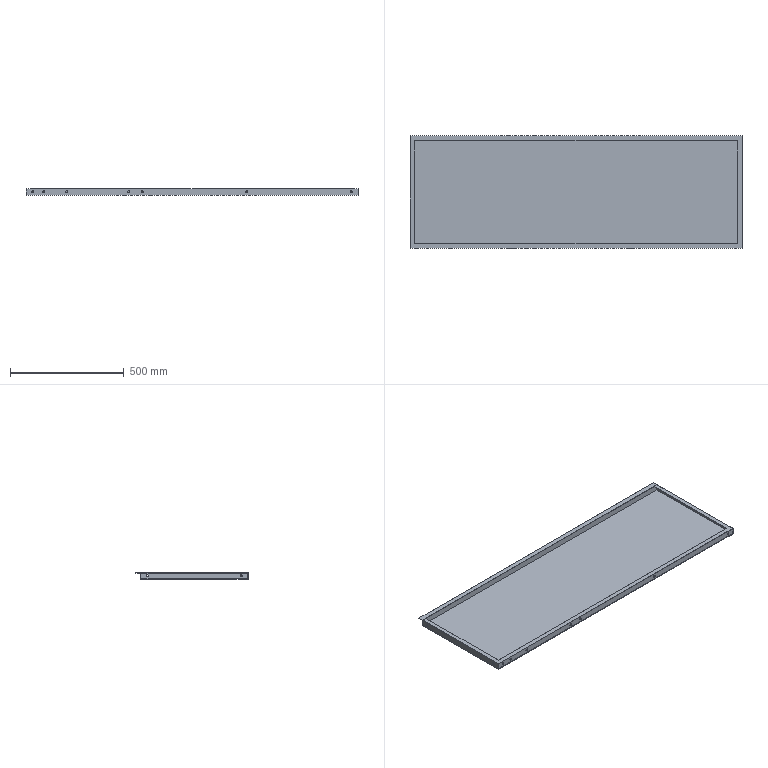Part | SolidWorks | features ICE 3, Extrusion 1, Shell 1 | 1 solid | 39 faces | box 1457 x 492 x 30 mm | volume 1732596 mm3 | cylinder 22 | plane 17 | commonest cylinder face diameters 9 x22
STEP:
#1=CARTESIAN_POINT('',(178.,0.,11.5));
#2=VERTEX_POINT('',#1);
#3=CARTESIAN_POINT('',(178.,0.,20.5));
#4=VERTEX_POINT('',#3);
#5=CARTESIAN_POINT('',(178.,0.,16.));
#6=DIRECTION('',(0.,1.,0.));
#7=DIRECTION('',(0.,0.,1.));
#8=AXIS2_PLACEMENT_3D('',#5,#6,#7);
#9=CIRCLE('',#8,4.5);
#10=EDGE_CURVE('',#2,#4,#9,.T.);
#11=ORIENTED_EDGE('',*,*,#10,.F.);
#12=CARTESIAN_POINT('',(178.,2.,11.5));
#13=VERTEX_POINT('',#12);
#14=CARTESIAN_POINT('',(178.,-8.,11.5));
#15=DIRECTION('',(0.,1.,0.));
#16=VECTOR('',#15,1000.);
#17=LINE('',#14,#16);
#18=EDGE_CURVE('',#2,#13,#17,.T.);
#19=ORIENTED_EDGE('',*,*,#18,.T.);
#20=CARTESIAN_POINT('',(178.,2.,20.5));
#21=VERTEX_POINT('',#20);
#22=CARTESIAN_POINT('',(178.,2.,16.));
#23=DIRECTION('',(0.,1.,0.));
#24=DIRECTION('',(0.,0.,1.));
#25=AXIS2_PLACEMENT_3D('',#22,#23,#24);
#26=CIRCLE('',#25,4.5);
#27=EDGE_CURVE('',#13,#21,#26,.T.);
#28=ORIENTED_EDGE('',*,*,#27,.T.);
#29=CARTESIAN_POINT('',(178.,-8.,20.5));
#30=DIRECTION('',(0.,1.,0.));
#31=VECTOR('',#30,1000.);
#32=LINE('',#29,#31);
#33=EDGE_CURVE('',#4,#21,#32,.T.);
#34=ORIENTED_EDGE('',*,*,#33,.F.);
#35=EDGE_LOOP('',(#11,#19,#28,#34));
#36=FACE_OUTER_BOUND('',#35,.T.);
#37=CARTESIAN_POINT('',(178.,-8.,16.));
#38=DIRECTION('',(0.,1.,0.));
#39=DIRECTION('',(0.,0.,1.));
#40=AXIS2_PLACEMENT_3D('',#37,#38,#39);
#41=CYLINDRICAL_SURFACE('',#40,4.5);
#42=ADVANCED_FACE('',(#36),#41,.F.);
#43=CARTESIAN_POINT('',(78.,0.,11.5));
#44=VERTEX_POINT('',#43);
#45=CARTESIAN_POINT('',(78.,0.,20.5));
#46=VERTEX_POINT('',#45);
#47=CARTESIAN_POINT('',(78.,0.,16.));
#48=DIRECTION('',(0.,1.,0.));
#49=DIRECTION('',(0.,0.,1.));
#50=AXIS2_PLACEMENT_3D('',#47,#48,#49);
#51=CIRCLE('',#50,4.5);
#52=EDGE_CURVE('',#44,#46,#51,.T.);
#53=ORIENTED_EDGE('',*,*,#52,.F.);
#54=CARTESIAN_POINT('',(78.,2.,11.5));
#55=VERTEX_POINT('',#54);
#56=CARTESIAN_POINT('',(78.,-8.,11.5));
#57=DIRECTION('',(0.,1.,0.));
#58=VECTOR('',#57,1000.);
#59=LINE('',#56,#58);
#60=EDGE_CURVE('',#44,#55,#59,.T.);
#61=ORIENTED_EDGE('',*,*,#60,.T.);
#62=CARTESIAN_POINT('',(78.,2.,20.5));
#63=VERTEX_POINT('',#62);
#64=CARTESIAN_POINT('',(78.,2.,16.));
#65=DIRECTION('',(0.,1.,0.));
#66=DIRECTION('',(0.,0.,1.));
#67=AXIS2_PLACEMENT_3D('',#64,#65,#66);
#68=CIRCLE('',#67,4.5);
#69=EDGE_CURVE('',#55,#63,#68,.T.);
#70=ORIENTED_EDGE('',*,*,#69,.T.);
#71=CARTESIAN_POINT('',(78.,-8.,20.5));
#72=DIRECTION('',(0.,1.,0.));
#73=VECTOR('',#72,1000.);
#74=LINE('',#71,#73);
#75=EDGE_CURVE('',#46,#63,#74,.T.);
#76=ORIENTED_EDGE('',*,*,#75,.F.);
#77=EDGE_LOOP('',(#53,#61,#70,#76));
#78=FACE_OUTER_BOUND('',#77,.T.);
#79=CARTESIAN_POINT('',(78.,-8.,16.));
#80=DIRECTION('',(0.,1.,0.));
#81=DIRECTION('',(0.,0.,1.));
#82=AXIS2_PLACEMENT_3D('',#79,#80,#81);
#83=CYLINDRICAL_SURFACE('',#82,4.5);
#84=ADVANCED_FACE('',(#78),#83,.F.);
#85=CARTESIAN_POINT('',(510.,0.,11.5));
#86=VERTEX_POINT('',#85);
#87=CARTESIAN_POINT('',(510.,0.,20.5));
#88=VERTEX_POINT('',#87);
#89=CARTESIAN_POINT('',(510.,0.,16.));
#90=DIRECTION('',(0.,1.,0.));
#91=DIRECTION('',(0.,0.,1.));
#92=AXIS2_PLACEMENT_3D('',#89,#90,#91);
#93=CIRCLE('',#92,4.5);
#94=EDGE_CURVE('',#86,#88,#93,.T.);
#95=ORIENTED_EDGE('',*,*,#94,.F.);
#96=CARTESIAN_POINT('',(510.,2.,11.5));
#97=VERTEX_POINT('',#96);
#98=CARTESIAN_POINT('',(510.,-8.,11.5));
#99=DIRECTION('',(0.,1.,0.));
#100=VECTOR('',#99,1000.);
#101=LINE('',#98,#100);
#102=EDGE_CURVE('',#86,#97,#101,.T.);
#103=ORIENTED_EDGE('',*,*,#102,.T.);
#104=CARTESIAN_POINT('',(510.,2.,20.5));
#105=VERTEX_POINT('',#104);
#106=CARTESIAN_POINT('',(510.,2.,16.));
#107=DIRECTION('',(0.,1.,0.));
#108=DIRECTION('',(0.,0.,1.));
#109=AXIS2_PLACEMENT_3D('',#106,#107,#108);
#110=CIRCLE('',#109,4.5);
#111=EDGE_CURVE('',#97,#105,#110,.T.);
#112=ORIENTED_EDGE('',*,*,#111,.T.);
#113=CARTESIAN_POINT('',(510.,-8.,20.5));
#114=DIRECTION('',(0.,1.,0.));
#115=VECTOR('',#114,1000.);
#116=LINE('',#113,#115);
#117=EDGE_CURVE('',#88,#105,#116,.T.);
#118=ORIENTED_EDGE('',*,*,#117,.F.);
#119=EDGE_LOOP('',(#95,#103,#112,#118));
#120=FACE_OUTER_BOUND('',#119,.T.);
#121=CARTESIAN_POINT('',(510.,-8.,16.));
#122=DIRECTION('',(0.,1.,0.));
#123=DIRECTION('',(0.,0.,1.));
#124=AXIS2_PLACEMENT_3D('',#121,#122,#123);
#125=CYLINDRICAL_SURFACE('',#124,4.5);
#126=ADVANCED_FACE('',(#120),#125,.F.);
#127=CARTESIAN_POINT('',(968.5,0.,11.5));
#128=VERTEX_POINT('',#127);
#129=CARTESIAN_POINT('',(968.5,0.,20.5));
#130=VERTEX_POINT('',#129);
#131=CARTESIAN_POINT('',(968.5,0.,16.));
#132=DIRECTION('',(0.,1.,0.));
#133=DIRECTION('',(0.,0.,1.));
#134=AXIS2_PLACEMENT_3D('',#131,#132,#133);
#135=CIRCLE('',#134,4.5);
#136=EDGE_CURVE('',#128,#130,#135,.T.);
#137=ORIENTED_EDGE('',*,*,#136,.F.);
#138=CARTESIAN_POINT('',(968.5,2.,11.5));
#139=VERTEX_POINT('',#138);
#140=CARTESIAN_POINT('',(968.5,-8.,11.5));
#141=DIRECTION('',(0.,1.,0.));
#142=VECTOR('',#141,1000.);
#143=LINE('',#140,#142);
#144=EDGE_CURVE('',#128,#139,#143,.T.);
#145=ORIENTED_EDGE('',*,*,#144,.T.);
#146=CARTESIAN_POINT('',(968.5,2.,20.5));
#147=VERTEX_POINT('',#146);
#148=CARTESIAN_POINT('',(968.5,2.,16.));
#149=DIRECTION('',(0.,1.,0.));
#150=DIRECTION('',(0.,0.,1.));
#151=AXIS2_PLACEMENT_3D('',#148,#149,#150);
#152=CIRCLE('',#151,4.5);
#153=EDGE_CURVE('',#139,#147,#152,.T.);
#154=ORIENTED_EDGE('',*,*,#153,.T.);
#155=CARTESIAN_POINT('',(968.5,-8.,20.5));
#156=DIRECTION('',(0.,1.,0.));
#157=VECTOR('',#156,1000.);
#158=LINE('',#155,#157);
#159=EDGE_CURVE('',#130,#147,#158,.T.);
#160=ORIENTED_EDGE('',*,*,#159,.F.);
#161=EDGE_LOOP('',(#137,#145,#154,#160));
#162=FACE_OUTER_BOUND('',#161,.T.);
#163=CARTESIAN_POINT('',(968.5,-8.,16.));
#164=DIRECTION('',(0.,1.,0.));
#165=DIRECTION('',(0.,0.,1.));
#166=AXIS2_PLACEMENT_3D('',#163,#164,#165);
#167=CYLINDRICAL_SURFACE('',#166,4.5);
#168=ADVANCED_FACE('',(#162),#167,.F.);
#169=CARTESIAN_POINT('',(1427.,0.,11.5));
#170=VERTEX_POINT('',#169);
#171=CARTESIAN_POINT('',(1427.,0.,20.5));
#172=VERTEX_POINT('',#171);
#173=CARTESIAN_POINT('',(1427.,0.,16.));
#174=DIRECTION('',(0.,1.,0.));
#175=DIRECTION('',(0.,0.,1.));
#176=AXIS2_PLACEMENT_3D('',#173,#174,#175);
#177=CIRCLE('',#176,4.5);
#178=EDGE_CURVE('',#170,#172,#177,.T.);
#179=ORIENTED_EDGE('',*,*,#178,.F.);
#180=CARTESIAN_POINT('',(1427.,2.,11.5));
#181=VERTEX_POINT('',#180);
#182=CARTESIAN_POINT('',(1427.,-8.,11.5));
#183=DIRECTION('',(0.,1.,0.));
#184=VECTOR('',#183,1000.);
#185=LINE('',#182,#184);
#186=EDGE_CURVE('',#170,#181,#185,.T.);
#187=ORIENTED_EDGE('',*,*,#186,.T.);
#188=CARTESIAN_POINT('',(1427.,2.,20.5));
#189=VERTEX_POINT('',#188);
#190=CARTESIAN_POINT('',(1427.,2.,16.));
#191=DIRECTION('',(0.,1.,0.));
#192=DIRECTION('',(0.,0.,1.));
#193=AXIS2_PLACEMENT_3D('',#190,#191,#192);
#194=CIRCLE('',#193,4.5);
#195=EDGE_CURVE('',#181,#189,#194,.T.);
#196=ORIENTED_EDGE('',*,*,#195,.T.);
#197=CARTESIAN_POINT('',(1427.,-8.,20.5));
#198=DIRECTION('',(0.,1.,0.));
#199=VECTOR('',#198,1000.);
#200=LINE('',#197,#199);
#201=EDGE_CURVE('',#172,#189,#200,.T.);
#202=ORIENTED_EDGE('',*,*,#201,.F.);
#203=EDGE_LOOP('',(#179,#187,#196,#202));
#204=FACE_OUTER_BOUND('',#203,.T.);
#205=CARTESIAN_POINT('',(1427.,-8.,16.));
#206=DIRECTION('',(0.,1.,0.));
#207=DIRECTION('',(0.,0.,1.));
#208=AXIS2_PLACEMENT_3D('',#205,#206,#207);
#209=CYLINDRICAL_SURFACE('',#208,4.5);
#210=ADVANCED_FACE('',(#204),#209,.F.);
#211=CARTESIAN_POINT('',(450.,0.,11.5));
#212=VERTEX_POINT('',#211);
#213=CARTESIAN_POINT('',(450.,0.,20.5));
#214=VERTEX_POINT('',#213);
#215=CARTESIAN_POINT('',(450.,0.,16.));
#216=DIRECTION('',(0.,1.,0.));
#217=DIRECTION('',(0.,0.,1.));
#218=AXIS2_PLACEMENT_3D('',#215,#216,#217);
#219=CIRCLE('',#218,4.5);
#220=EDGE_CURVE('',#212,#214,#219,.T.);
#221=ORIENTED_EDGE('',*,*,#220,.F.);
#222=CARTESIAN_POINT('',(450.,2.,11.5));
#223=VERTEX_POINT('',#222);
#224=CARTESIAN_POINT('',(450.,-8.,11.5));
#225=DIRECTION('',(0.,1.,0.));
#226=VECTOR('',#225,1000.);
#227=LINE('',#224,#226);
#228=EDGE_CURVE('',#212,#223,#227,.T.);
#229=ORIENTED_EDGE('',*,*,#228,.T.);
#230=CARTESIAN_POINT('',(450.,2.,20.5));
#231=VERTEX_POINT('',#230);
#232=CARTESIAN_POINT('',(450.,2.,16.));
#233=DIRECTION('',(0.,1.,0.));
#234=DIRECTION('',(0.,0.,1.));
#235=AXIS2_PLACEMENT_3D('',#232,#233,#234);
#236=CIRCLE('',#235,4.5);
#237=EDGE_CURVE('',#223,#231,#236,.T.);
#238=ORIENTED_EDGE('',*,*,#237,.T.);
#239=CARTESIAN_POINT('',(450.,-8.,20.5));
#240=DIRECTION('',(0.,1.,0.));
#241=VECTOR('',#240,1000.);
#242=LINE('',#239,#241);
#243=EDGE_CURVE('',#214,#231,#242,.T.);
#244=ORIENTED_EDGE('',*,*,#243,.F.);
#245=EDGE_LOOP('',(#221,#229,#238,#244));
#246=FACE_OUTER_BOUND('',#245,.T.);
#247=CARTESIAN_POINT('',(450.,-8.,16.));
#248=DIRECTION('',(0.,1.,0.));
#249=DIRECTION('',(0.,0.,1.));
#250=AXIS2_PLACEMENT_3D('',#247,#248,#249);
#251=CYLINDRICAL_SURFACE('',#250,4.5);
#252=ADVANCED_FACE('',(#246),#251,.F.);
#253=CARTESIAN_POINT('',(30.,0.,11.5));
#254=VERTEX_POINT('',#253);
#255=CARTESIAN_POINT('',(30.,0.,20.5));
#256=VERTEX_POINT('',#255);
#257=CARTESIAN_POINT('',(30.,0.,16.));
#258=DIRECTION('',(0.,1.,0.));
#259=DIRECTION('',(0.,0.,1.));
#260=AXIS2_PLACEMENT_3D('',#257,#258,#259);
#261=CIRCLE('',#260,4.5);
#262=EDGE_CURVE('',#254,#256,#261,.T.);
#263=ORIENTED_EDGE('',*,*,#262,.F.);
#264=CARTESIAN_POINT('',(30.,2.,11.5));
#265=VERTEX_POINT('',#264);
#266=CARTESIAN_POINT('',(30.,-8.,11.5));
#267=DIRECTION('',(0.,1.,0.));
#268=VECTOR('',#267,1000.);
#269=LINE('',#266,#268);
#270=EDGE_CURVE('',#254,#265,#269,.T.);
#271=ORIENTED_EDGE('',*,*,#270,.T.);
#272=CARTESIAN_POINT('',(30.,2.,20.5));
#273=VERTEX_POINT('',#272);
#274=CARTESIAN_POINT('',(30.,2.,16.));
#275=DIRECTION('',(0.,1.,0.));
#276=DIRECTION('',(0.,0.,1.));
#277=AXIS2_PLACEMENT_3D('',#274,#275,#276);
#278=CIRCLE('',#277,4.5);
#279=EDGE_CURVE('',#265,#273,#278,.T.);
#280=ORIENTED_EDGE('',*,*,#279,.T.);
#281=CARTESIAN_POINT('',(30.,-8.,20.5));
#282=DIRECTION('',(0.,1.,0.));
#283=VECTOR('',#282,1000.);
#284=LINE('',#281,#283);
#285=EDGE_CURVE('',#256,#273,#284,.T.);
#286=ORIENTED_EDGE('',*,*,#285,.F.);
#287=EDGE_LOOP('',(#263,#271,#280,#286));
#288=FACE_OUTER_BOUND('',#287,.T.);
#289=CARTESIAN_POINT('',(30.,-8.,16.));
#290=DIRECTION('',(0.,1.,0.));
#291=DIRECTION('',(0.,0.,1.));
#292=AXIS2_PLACEMENT_3D('',#289,#290,#291);
#293=CYLINDRICAL_SURFACE('',#292,4.5);
#294=ADVANCED_FACE('',(#288),#293,.F.);
#295=CARTESIAN_POINT('',(2.,30.,11.5));
#296=VERTEX_POINT('',#295);
#297=CARTESIAN_POINT('',(2.,30.,20.5));
#298=VERTEX_POINT('',#297);
#299=CARTESIAN_POINT('',(2.,30.,16.));
#300=DIRECTION('',(-1.,0.,0.));
#301=DIRECTION('',(0.,0.,-1.));
#302=AXIS2_PLACEMENT_3D('',#299,#300,#301);
#303=CIRCLE('',#302,4.5);
#304=EDGE_CURVE('',#296,#298,#303,.T.);
#305=ORIENTED_EDGE('',*,*,#304,.F.);
#306=CARTESIAN_POINT('',(0.,30.,11.5));
#307=VERTEX_POINT('',#306);
#308=CARTESIAN_POINT('',(1503.,30.,11.5));
#309=DIRECTION('',(-1.,0.,0.));
#310=VECTOR('',#309,1000.);
#311=LINE('',#308,#310);
#312=EDGE_CURVE('',#296,#307,#311,.T.);
#313=ORIENTED_EDGE('',*,*,#312,.T.);
#314=CARTESIAN_POINT('',(0.,30.,20.5));
#315=VERTEX_POINT('',#314);
#316=CARTESIAN_POINT('',(0.,30.,16.));
#317=DIRECTION('',(-1.,0.,0.));
#318=DIRECTION('',(0.,0.,-1.));
#319=AXIS2_PLACEMENT_3D('',#316,#317,#318);
#320=CIRCLE('',#319,4.5);
#321=EDGE_CURVE('',#307,#315,#320,.T.);
#322=ORIENTED_EDGE('',*,*,#321,.T.);
#323=CARTESIAN_POINT('',(1503.,30.,20.5));
#324=DIRECTION('',(-1.,0.,0.));
#325=VECTOR('',#324,1000.);
#326=LINE('',#323,#325);
#327=EDGE_CURVE('',#298,#315,#326,.T.);
#328=ORIENTED_EDGE('',*,*,#327,.F.);
#329=EDGE_LOOP('',(#305,#313,#322,#328));
#330=FACE_OUTER_BOUND('',#329,.T.);
#331=CARTESIAN_POINT('',(1503.,30.,16.));
#332=DIRECTION('',(-1.,0.,0.));
#333=DIRECTION('',(0.,0.,1.));
#334=AXIS2_PLACEMENT_3D('',#331,#332,#333);
#335=CYLINDRICAL_SURFACE('',#334,4.5);
#336=ADVANCED_FACE('',(#330),#335,.F.);
#337=CARTESIAN_POINT('',(1457.,30.,20.5));
#338=VERTEX_POINT('',#337);
#339=CARTESIAN_POINT('',(1457.,30.,11.5));
#340=VERTEX_POINT('',#339);
#341=CARTESIAN_POINT('',(1457.,30.,16.));
#342=DIRECTION('',(1.,0.,0.));
#343=DIRECTION('',(0.,0.,1.));
#344=AXIS2_PLACEMENT_3D('',#341,#342,#343);
#345=CIRCLE('',#344,4.5);
#346=EDGE_CURVE('',#338,#340,#345,.T.);
#347=ORIENTED_EDGE('',*,*,#346,.T.);
#348=CARTESIAN_POINT('',(1455.,30.,11.5));
#349=VERTEX_POINT('',#348);
#350=CARTESIAN_POINT('',(1503.,30.,11.5));
#351=DIRECTION('',(-1.,0.,0.));
#352=VECTOR('',#351,1000.);
#353=LINE('',#350,#352);
#354=EDGE_CURVE('',#340,#349,#353,.T.);
#355=ORIENTED_EDGE('',*,*,#354,.T.);
#356=CARTESIAN_POINT('',(1455.,30.,20.5));
#357=VERTEX_POINT('',#356);
#358=CARTESIAN_POINT('',(1455.,30.,16.));
#359=DIRECTION('',(1.,0.,0.));
#360=DIRECTION('',(0.,0.,1.));
#361=AXIS2_PLACEMENT_3D('',#358,#359,#360);
#362=CIRCLE('',#361,4.5);
#363=EDGE_CURVE('',#357,#349,#362,.T.);
#364=ORIENTED_EDGE('',*,*,#363,.F.);
#365=CARTESIAN_POINT('',(1503.,30.,20.5));
#366=DIRECTION('',(-1.,0.,0.));
#367=VECTOR('',#366,1000.);
#368=LINE('',#365,#367);
#369=EDGE_CURVE('',#338,#357,#368,.T.);
#370=ORIENTED_EDGE('',*,*,#369,.F.);
#371=EDGE_LOOP('',(#347,#355,#364,#370));
#372=FACE_OUTER_BOUND('',#371,.T.);
#373=CARTESIAN_POINT('',(1503.,30.,16.));
#374=DIRECTION('',(-1.,0.,0.));
#375=DIRECTION('',(0.,0.,1.));
#376=AXIS2_PLACEMENT_3D('',#373,#374,#375);
#377=CYLINDRICAL_SURFACE('',#376,4.5);
#378=ADVANCED_FACE('',(#372),#377,.F.);
#379=CARTESIAN_POINT('',(2.,442.,11.5));
#380=VERTEX_POINT('',#379);
#381=CARTESIAN_POINT('',(2.,442.,20.5));
#382=VERTEX_POINT('',#381);
#383=CARTESIAN_POINT('',(2.,442.,16.));
#384=DIRECTION('',(-1.,0.,0.));
#385=DIRECTION('',(0.,0.,-1.));
#386=AXIS2_PLACEMENT_3D('',#383,#384,#385);
#387=CIRCLE('',#386,4.5);
#388=EDGE_CURVE('',#380,#382,#387,.T.);
#389=ORIENTED_EDGE('',*,*,#388,.F.);
#390=CARTESIAN_POINT('',(0.,442.,11.5));
#391=VERTEX_POINT('',#390);
#392=CARTESIAN_POINT('',(1503.,442.,11.5));
#393=DIRECTION('',(-1.,0.,0.));
#394=VECTOR('',#393,1000.);
#395=LINE('',#392,#394);
#396=EDGE_CURVE('',#380,#391,#395,.T.);
#397=ORIENTED_EDGE('',*,*,#396,.T.);
#398=CARTESIAN_POINT('',(0.,442.,20.5));
#399=VERTEX_POINT('',#398);
#400=CARTESIAN_POINT('',(0.,442.,16.));
#401=DIRECTION('',(-1.,0.,0.));
#402=DIRECTION('',(0.,0.,-1.));
#403=AXIS2_PLACEMENT_3D('',#400,#401,#402);
#404=CIRCLE('',#403,4.5);
#405=EDGE_CURVE('',#391,#399,#404,.T.);
#406=ORIENTED_EDGE('',*,*,#405,.T.);
#407=CARTESIAN_POINT('',(1503.,442.,20.5));
#408=DIRECTION('',(-1.,0.,0.));
#409=VECTOR('',#408,1000.);
#410=LINE('',#407,#409);
#411=EDGE_CURVE('',#382,#399,#410,.T.);
#412=ORIENTED_EDGE('',*,*,#411,.F.);
#413=EDGE_LOOP('',(#389,#397,#406,#412));
#414=FACE_OUTER_BOUND('',#413,.T.);
#415=CARTESIAN_POINT('',(1503.,442.,16.));
#416=DIRECTION('',(-1.,0.,0.));
#417=DIRECTION('',(0.,0.,1.));
#418=AXIS2_PLACEMENT_3D('',#415,#416,#417);
#419=CYLINDRICAL_SURFACE('',#418,4.5);
#420=ADVANCED_FACE('',(#414),#419,.F.);
#421=CARTESIAN_POINT('',(1457.,442.,20.5));
#422=VERTEX_POINT('',#421);
#423=CARTESIAN_POINT('',(1457.,442.,11.5));
#424=VERTEX_POINT('',#423);
#425=CARTESIAN_POINT('',(1457.,442.,16.));
#426=DIRECTION('',(1.,0.,0.));
#427=DIRECTION('',(0.,0.,1.));
#428=AXIS2_PLACEMENT_3D('',#425,#426,#427);
#429=CIRCLE('',#428,4.5);
#430=EDGE_CURVE('',#422,#424,#429,.T.);
#431=ORIENTED_EDGE('',*,*,#430,.T.);
#432=CARTESIAN_POINT('',(1455.,442.,11.5));
#433=VERTEX_POINT('',#432);
#434=CARTESIAN_POINT('',(1503.,442.,11.5));
#435=DIRECTION('',(-1.,0.,0.));
#436=VECTOR('',#435,1000.);
#437=LINE('',#434,#436);
#438=EDGE_CURVE('',#424,#433,#437,.T.);
#439=ORIENTED_EDGE('',*,*,#438,.T.);
#440=CARTESIAN_POINT('',(1455.,442.,20.5));
#441=VERTEX_POINT('',#440);
#442=CARTESIAN_POINT('',(1455.,442.,16.));
#443=DIRECTION('',(1.,0.,0.));
#444=DIRECTION('',(0.,0.,1.));
#445=AXIS2_PLACEMENT_3D('',#442,#443,#444);
#446=CIRCLE('',#445,4.5);
#447=EDGE_CURVE('',#441,#433,#446,.T.);
#448=ORIENTED_EDGE('',*,*,#447,.F.);
#449=CARTESIAN_POINT('',(1503.,442.,20.5));
#450=DIRECTION('',(-1.,0.,0.));
#451=VECTOR('',#450,1000.);
#452=LINE('',#449,#451);
#453=EDGE_CURVE('',#422,#441,#452,.T.);
#454=ORIENTED_EDGE('',*,*,#453,.F.);
#455=EDGE_LOOP('',(#431,#439,#448,#454));
#456=FACE_OUTER_BOUND('',#455,.T.);
#457=CARTESIAN_POINT('',(1503.,442.,16.));
#458=DIRECTION('',(-1.,0.,0.));
#459=DIRECTION('',(0.,0.,1.));
#460=AXIS2_PLACEMENT_3D('',#457,#458,#459);
#461=CYLINDRICAL_SURFACE('',#460,4.5);
#462=ADVANCED_FACE('',(#456),#461,.F.);
#463=CARTESIAN_POINT('',(2.,442.,16.));
#464=DIRECTION('',(-1.,0.,0.));
#465=DIRECTION('',(0.,0.,-1.));
#466=AXIS2_PLACEMENT_3D('',#463,#464,#465);
#467=CIRCLE('',#466,4.5);
#468=EDGE_CURVE('',#382,#380,#467,.T.);
#469=ORIENTED_EDGE('',*,*,#468,.T.);
#470=ORIENTED_EDGE('',*,*,#388,.T.);
#471=EDGE_LOOP('',(#469,#470));
#472=FACE_BOUND('',#471,.T.);
#473=CARTESIAN_POINT('',(2.,470.,28.));
#474=VERTEX_POINT('',#473);
#475=CARTESIAN_POINT('',(2.,470.,2.));
#476=VERTEX_POINT('',#475);
#477=CARTESIAN_POINT('',(2.,470.,30.));
#478=DIRECTION('',(0.,0.,-1.));
#479=VECTOR('',#478,1000.);
#480=LINE('',#477,#479);
#481=EDGE_CURVE('',#474,#476,#480,.T.);
#482=ORIENTED_EDGE('',*,*,#481,.F.);
#483=CARTESIAN_POINT('',(2.,2.,28.));
#484=VERTEX_POINT('',#483);
#485=CARTESIAN_POINT('',(2.,0.,28.));
#486=DIRECTION('',(0.,-1.,0.));
#487=VECTOR('',#486,1000.);
#488=LINE('',#485,#487);
#489=EDGE_CURVE('',#474,#484,#488,.T.);
#490=ORIENTED_EDGE('',*,*,#489,.T.);
#491=CARTESIAN_POINT('',(2.,2.,2.));
#492=VERTEX_POINT('',#491);
#493=CARTESIAN_POINT('',(2.,2.,30.));
#494=DIRECTION('',(0.,0.,-1.));
#495=VECTOR('',#494,1000.);
#496=LINE('',#493,#495);
#497=EDGE_CURVE('',#484,#492,#496,.T.);
#498=ORIENTED_EDGE('',*,*,#497,.T.);
#499=CARTESIAN_POINT('',(2.,472.,2.));
#500=DIRECTION('',(0.,-1.,0.));
#501=VECTOR('',#500,1000.);
#502=LINE('',#499,#501);
#503=EDGE_CURVE('',#476,#492,#502,.T.);
#504=ORIENTED_EDGE('',*,*,#503,.F.);
#505=EDGE_LOOP('',(#482,#490,#498,#504));
#506=FACE_OUTER_BOUND('',#505,.T.);
#507=CARTESIAN_POINT('',(2.,30.,16.));
#508=DIRECTION('',(-1.,0.,0.));
#509=DIRECTION('',(0.,0.,-1.));
#510=AXIS2_PLACEMENT_3D('',#507,#508,#509);
#511=CIRCLE('',#510,4.5);
#512=EDGE_CURVE('',#298,#296,#511,.T.);
#513=ORIENTED_EDGE('',*,*,#512,.T.);
#514=ORIENTED_EDGE('',*,*,#304,.T.);
#515=EDGE_LOOP('',(#513,#514));
#516=FACE_BOUND('',#515,.T.);
#517=CARTESIAN_POINT('',(2.,0.,30.));
#518=DIRECTION('',(1.,0.,0.));
#519=DIRECTION('',(0.,0.,-1.));
#520=AXIS2_PLACEMENT_3D('',#517,#518,#519);
#521=PLANE('',#520);
#522=ADVANCED_FACE('',(#472,#506,#516),#521,.T.);
#523=ORIENTED_EDGE('',*,*,#447,.T.);
#524=CARTESIAN_POINT('',(1455.,442.,16.));
#525=DIRECTION('',(1.,0.,0.));
#526=DIRECTION('',(0.,0.,1.));
#527=AXIS2_PLACEMENT_3D('',#524,#525,#526);
#528=CIRCLE('',#527,4.5);
#529=EDGE_CURVE('',#433,#441,#528,.T.);
#530=ORIENTED_EDGE('',*,*,#529,.T.);
#531=EDGE_LOOP('',(#523,#530));
#532=FACE_BOUND('',#531,.T.);
#533=CARTESIAN_POINT('',(1455.,2.,28.));
#534=VERTEX_POINT('',#533);
#535=CARTESIAN_POINT('',(1455.,2.,2.));
#536=VERTEX_POINT('',#535);
#537=CARTESIAN_POINT('',(1455.,2.,30.));
#538=DIRECTION('',(0.,0.,-1.));
#539=VECTOR('',#538,1000.);
#540=LINE('',#537,#539);
#541=EDGE_CURVE('',#534,#536,#540,.T.);
#542=ORIENTED_EDGE('',*,*,#541,.F.);
#543=CARTESIAN_POINT('',(1455.,470.,28.));
#544=VERTEX_POINT('',#543);
#545=CARTESIAN_POINT('',(1455.,0.,28.));
#546=DIRECTION('',(0.,1.,0.));
#547=VECTOR('',#546,1000.);
#548=LINE('',#545,#547);
#549=EDGE_CURVE('',#534,#544,#548,.T.);
#550=ORIENTED_EDGE('',*,*,#549,.T.);
#551=CARTESIAN_POINT('',(1455.,470.,2.));
#552=VERTEX_POINT('',#551);
#553=CARTESIAN_POINT('',(1455.,470.,30.));
#554=DIRECTION('',(0.,0.,-1.));
#555=VECTOR('',#554,1000.);
#556=LINE('',#553,#555);
#557=EDGE_CURVE('',#544,#552,#556,.T.);
#558=ORIENTED_EDGE('',*,*,#557,.T.);
#559=CARTESIAN_POINT('',(1455.,472.,2.));
#560=DIRECTION('',(0.,1.,0.));
#561=VECTOR('',#560,1000.);
#562=LINE('',#559,#561);
#563=EDGE_CURVE('',#536,#552,#562,.T.);
#564=ORIENTED_EDGE('',*,*,#563,.F.);
#565=EDGE_LOOP('',(#542,#550,#558,#564));
#566=FACE_OUTER_BOUND('',#565,.T.);
#567=ORIENTED_EDGE('',*,*,#363,.T.);
#568=CARTESIAN_POINT('',(1455.,30.,16.));
#569=DIRECTION('',(1.,0.,0.));
#570=DIRECTION('',(0.,0.,1.));
#571=AXIS2_PLACEMENT_3D('',#568,#569,#570);
#572=CIRCLE('',#571,4.5);
#573=EDGE_CURVE('',#349,#357,#572,.T.);
#574=ORIENTED_EDGE('',*,*,#573,.T.);
#575=EDGE_LOOP('',(#567,#574));
#576=FACE_BOUND('',#575,.T.);
#577=CARTESIAN_POINT('',(1455.,0.,30.));
#578=DIRECTION('',(-1.,0.,0.));
#579=DIRECTION('',(0.,0.,1.));
#580=AXIS2_PLACEMENT_3D('',#577,#578,#579);
#581=PLANE('',#580);
#582=ADVANCED_FACE('',(#532,#566,#576),#581,.T.);
#583=CARTESIAN_POINT('',(0.,442.,16.));
#584=DIRECTION('',(-1.,0.,0.));
#585=DIRECTION('',(0.,0.,-1.));
#586=AXIS2_PLACEMENT_3D('',#583,#584,#585);
#587=CIRCLE('',#586,4.5);
#588=EDGE_CURVE('',#399,#391,#587,.T.);
#589=ORIENTED_EDGE('',*,*,#588,.F.);
#590=ORIENTED_EDGE('',*,*,#405,.F.);
#591=EDGE_LOOP('',(#589,#590));
#592=FACE_BOUND('',#591,.T.);
#593=CARTESIAN_POINT('',(0.,492.,30.));
#594=VERTEX_POINT('',#593);
#595=CARTESIAN_POINT('',(0.,0.,30.));
#596=VERTEX_POINT('',#595);
#597=CARTESIAN_POINT('',(0.,0.,30.));
#598=DIRECTION('',(0.,-1.,0.));
#599=VECTOR('',#598,1000.);
#600=LINE('',#597,#599);
#601=EDGE_CURVE('',#594,#596,#600,.T.);
#602=ORIENTED_EDGE('',*,*,#601,.F.);
#603=CARTESIAN_POINT('',(0.,492.,28.));
#604=VERTEX_POINT('',#603);
#605=CARTESIAN_POINT('',(0.,492.,28.));
#606=DIRECTION('',(0.,0.,1.));
#607=VECTOR('',#606,1000.);
#608=LINE('',#605,#607);
#609=EDGE_CURVE('',#604,#594,#608,.T.);
#610=ORIENTED_EDGE('',*,*,#609,.F.);
#611=CARTESIAN_POINT('',(0.,472.,28.));
#612=VERTEX_POINT('',#611);
#613=CARTESIAN_POINT('',(0.,492.,28.));
#614=DIRECTION('',(0.,-1.,0.));
#615=VECTOR('',#614,1000.);
#616=LINE('',#613,#615);
#617=EDGE_CURVE('',#604,#612,#616,.T.);
#618=ORIENTED_EDGE('',*,*,#617,.T.);
#619=CARTESIAN_POINT('',(0.,472.,0.));
#620=VERTEX_POINT('',#619);
#621=CARTESIAN_POINT('',(0.,472.,30.));
#622=DIRECTION('',(0.,0.,-1.));
#623=VECTOR('',#622,1000.);
#624=LINE('',#621,#623);
#625=EDGE_CURVE('',#612,#620,#624,.T.);
#626=ORIENTED_EDGE('',*,*,#625,.T.);
#627=CARTESIAN_POINT('',(0.,0.,0.));
#628=VERTEX_POINT('',#627);
#629=CARTESIAN_POINT('',(0.,0.,0.));
#630=DIRECTION('',(0.,-1.,0.));
#631=VECTOR('',#630,1000.);
#632=LINE('',#629,#631);
#633=EDGE_CURVE('',#620,#628,#632,.T.);
#634=ORIENTED_EDGE('',*,*,#633,.T.);
#635=CARTESIAN_POINT('',(0.,0.,30.));
#636=DIRECTION('',(0.,0.,-1.));
#637=VECTOR('',#636,1000.);
#638=LINE('',#635,#637);
#639=EDGE_CURVE('',#596,#628,#638,.T.);
#640=ORIENTED_EDGE('',*,*,#639,.F.);
#641=EDGE_LOOP('',(#602,#610,#618,#626,#634,#640));
#642=FACE_OUTER_BOUND('',#641,.T.);
#643=CARTESIAN_POINT('',(0.,30.,16.));
#644=DIRECTION('',(-1.,0.,0.));
#645=DIRECTION('',(0.,0.,-1.));
#646=AXIS2_PLACEMENT_3D('',#643,#644,#645);
#647=CIRCLE('',#646,4.5);
#648=EDGE_CURVE('',#315,#307,#647,.T.);
#649=ORIENTED_EDGE('',*,*,#648,.F.);
#650=ORIENTED_EDGE('',*,*,#321,.F.);
#651=EDGE_LOOP('',(#649,#650));
#652=FACE_BOUND('',#651,.T.);
#653=CARTESIAN_POINT('',(0.,0.,30.));
#654=DIRECTION('',(1.,0.,0.));
#655=DIRECTION('',(0.,0.,-1.));
#656=AXIS2_PLACEMENT_3D('',#653,#654,#655);
#657=PLANE('',#656);
#658=ADVANCED_FACE('',(#592,#642,#652),#657,.F.);
#659=ORIENTED_EDGE('',*,*,#430,.F.);
#660=CARTESIAN_POINT('',(1457.,442.,16.));
#661=DIRECTION('',(1.,0.,0.));
#662=DIRECTION('',(0.,0.,1.));
#663=AXIS2_PLACEMENT_3D('',#660,#661,#662);
#664=CIRCLE('',#663,4.5);
#665=EDGE_CURVE('',#424,#422,#664,.T.);
#666=ORIENTED_EDGE('',*,*,#665,.F.);
#667=EDGE_LOOP('',(#659,#666));
#668=FACE_BOUND('',#667,.T.);
#669=CARTESIAN_POINT('',(1457.,0.,30.));
#670=VERTEX_POINT('',#669);
#671=CARTESIAN_POINT('',(1457.,0.,0.));
#672=VERTEX_POINT('',#671);
#673=CARTESIAN_POINT('',(1457.,0.,30.));
#674=DIRECTION('',(0.,0.,-1.));
#675=VECTOR('',#674,1000.);
#676=LINE('',#673,#675);
#677=EDGE_CURVE('',#670,#672,#676,.T.);
#678=ORIENTED_EDGE('',*,*,#677,.T.);
#679=CARTESIAN_POINT('',(1457.,472.,0.));
#680=VERTEX_POINT('',#679);
#681=CARTESIAN_POINT('',(1457.,0.,0.));
#682=DIRECTION('',(0.,1.,0.));
#683=VECTOR('',#682,1000.);
#684=LINE('',#681,#683);
#685=EDGE_CURVE('',#672,#680,#684,.T.);
#686=ORIENTED_EDGE('',*,*,#685,.T.);
#687=CARTESIAN_POINT('',(1457.,472.,28.));
#688=VERTEX_POINT('',#687);
#689=CARTESIAN_POINT('',(1457.,472.,30.));
#690=DIRECTION('',(0.,0.,-1.));
#691=VECTOR('',#690,1000.);
#692=LINE('',#689,#691);
#693=EDGE_CURVE('',#688,#680,#692,.T.);
#694=ORIENTED_EDGE('',*,*,#693,.F.);
#695=CARTESIAN_POINT('',(1457.,492.,28.));
#696=VERTEX_POINT('',#695);
#697=CARTESIAN_POINT('',(1457.,492.,28.));
#698=DIRECTION('',(0.,1.,0.));
#699=VECTOR('',#698,1000.);
#700=LINE('',#697,#699);
#701=EDGE_CURVE('',#688,#696,#700,.T.);
#702=ORIENTED_EDGE('',*,*,#701,.T.);
#703=CARTESIAN_POINT('',(1457.,492.,30.));
#704=VERTEX_POINT('',#703);
#705=CARTESIAN_POINT('',(1457.,492.,28.));
#706=DIRECTION('',(0.,0.,1.));
#707=VECTOR('',#706,1000.);
#708=LINE('',#705,#707);
#709=EDGE_CURVE('',#696,#704,#708,.T.);
#710=ORIENTED_EDGE('',*,*,#709,.T.);
#711=CARTESIAN_POINT('',(1457.,0.,30.));
#712=DIRECTION('',(0.,1.,0.));
#713=VECTOR('',#712,1000.);
#714=LINE('',#711,#713);
#715=EDGE_CURVE('',#670,#704,#714,.T.);
#716=ORIENTED_EDGE('',*,*,#715,.F.);
#717=EDGE_LOOP('',(#678,#686,#694,#702,#710,#716));
#718=FACE_OUTER_BOUND('',#717,.T.);
#719=ORIENTED_EDGE('',*,*,#346,.F.);
#720=CARTESIAN_POINT('',(1457.,30.,16.));
#721=DIRECTION('',(1.,0.,0.));
#722=DIRECTION('',(0.,0.,1.));
#723=AXIS2_PLACEMENT_3D('',#720,#721,#722);
#724=CIRCLE('',#723,4.5);
#725=EDGE_CURVE('',#340,#338,#724,.T.);
#726=ORIENTED_EDGE('',*,*,#725,.F.);
#727=EDGE_LOOP('',(#719,#726));
#728=FACE_BOUND('',#727,.T.);
#729=CARTESIAN_POINT('',(1457.,0.,30.));
#730=DIRECTION('',(-1.,0.,0.));
#731=DIRECTION('',(0.,0.,1.));
#732=AXIS2_PLACEMENT_3D('',#729,#730,#731);
#733=PLANE('',#732);
#734=ADVANCED_FACE('',(#668,#718,#728),#733,.F.);
#735=CARTESIAN_POINT('',(0.,472.,28.));
#736=DIRECTION('',(-1.,0.,0.));
#737=VECTOR('',#736,1000.);
#738=LINE('',#735,#737);
#739=EDGE_CURVE('',#688,#612,#738,.T.);
#740=ORIENTED_EDGE('',*,*,#739,.F.);
#741=ORIENTED_EDGE('',*,*,#693,.T.);
#742=CARTESIAN_POINT('',(0.,472.,0.));
#743=DIRECTION('',(-1.,0.,0.));
#744=VECTOR('',#743,1000.);
#745=LINE('',#742,#744);
#746=EDGE_CURVE('',#680,#620,#745,.T.);
#747=ORIENTED_EDGE('',*,*,#746,.T.);
#748=ORIENTED_EDGE('',*,*,#625,.F.);
#749=EDGE_LOOP('',(#740,#741,#747,#748));
#750=FACE_OUTER_BOUND('',#749,.T.);
#751=CARTESIAN_POINT('',(0.,472.,30.));
#752=DIRECTION('',(0.,-1.,0.));
#753=DIRECTION('',(1.,0.,0.));
#754=AXIS2_PLACEMENT_3D('',#751,#752,#753);
#755=PLANE('',#754);
#756=ADVANCED_FACE('',(#750),#755,.F.);
#757=CARTESIAN_POINT('',(178.,2.,16.));
#758=DIRECTION('',(0.,1.,0.));
#759=DIRECTION('',(0.,0.,1.));
#760=AXIS2_PLACEMENT_3D('',#757,#758,#759);
#761=CIRCLE('',#760,4.5);
#762=EDGE_CURVE('',#21,#13,#761,.T.);
#763=ORIENTED_EDGE('',*,*,#762,.F.);
#764=ORIENTED_EDGE('',*,*,#27,.F.);
#765=EDGE_LOOP('',(#763,#764));
#766=FACE_BOUND('',#765,.T.);
#767=CARTESIAN_POINT('',(78.,2.,16.));
#768=DIRECTION('',(0.,1.,0.));
#769=DIRECTION('',(0.,0.,1.));
#770=AXIS2_PLACEMENT_3D('',#767,#768,#769);
#771=CIRCLE('',#770,4.5);
#772=EDGE_CURVE('',#63,#55,#771,.T.);
#773=ORIENTED_EDGE('',*,*,#772,.F.);
#774=ORIENTED_EDGE('',*,*,#69,.F.);
#775=EDGE_LOOP('',(#773,#774));
#776=FACE_BOUND('',#775,.T.);
#777=CARTESIAN_POINT('',(510.,2.,16.));
#778=DIRECTION('',(0.,1.,0.));
#779=DIRECTION('',(0.,0.,1.));
#780=AXIS2_PLACEMENT_3D('',#777,#778,#779);
#781=CIRCLE('',#780,4.5);
#782=EDGE_CURVE('',#105,#97,#781,.T.);
#783=ORIENTED_EDGE('',*,*,#782,.F.);
#784=ORIENTED_EDGE('',*,*,#111,.F.);
#785=EDGE_LOOP('',(#783,#784));
#786=FACE_BOUND('',#785,.T.);
#787=CARTESIAN_POINT('',(968.5,2.,16.));
#788=DIRECTION('',(0.,1.,0.));
#789=DIRECTION('',(0.,0.,1.));
#790=AXIS2_PLACEMENT_3D('',#787,#788,#789);
#791=CIRCLE('',#790,4.5);
#792=EDGE_CURVE('',#147,#139,#791,.T.);
#793=ORIENTED_EDGE('',*,*,#792,.F.);
#794=ORIENTED_EDGE('',*,*,#153,.F.);
#795=EDGE_LOOP('',(#793,#794));
#796=FACE_BOUND('',#795,.T.);
#797=CARTESIAN_POINT('',(1427.,2.,16.));
#798=DIRECTION('',(0.,1.,0.));
#799=DIRECTION('',(0.,0.,1.));
#800=AXIS2_PLACEMENT_3D('',#797,#798,#799);
#801=CIRCLE('',#800,4.5);
#802=EDGE_CURVE('',#189,#181,#801,.T.);
#803=ORIENTED_EDGE('',*,*,#802,.F.);
#804=ORIENTED_EDGE('',*,*,#195,.F.);
#805=EDGE_LOOP('',(#803,#804));
#806=FACE_BOUND('',#805,.T.);
#807=CARTESIAN_POINT('',(450.,2.,16.));
#808=DIRECTION('',(0.,1.,0.));
#809=DIRECTION('',(0.,0.,1.));
#810=AXIS2_PLACEMENT_3D('',#807,#808,#809);
#811=CIRCLE('',#810,4.5);
#812=EDGE_CURVE('',#231,#223,#811,.T.);
#813=ORIENTED_EDGE('',*,*,#812,.F.);
#814=ORIENTED_EDGE('',*,*,#237,.F.);
#815=EDGE_LOOP('',(#813,#814));
#816=FACE_BOUND('',#815,.T.);
#817=CARTESIAN_POINT('',(30.,2.,16.));
#818=DIRECTION('',(0.,1.,0.));
#819=DIRECTION('',(0.,0.,1.));
#820=AXIS2_PLACEMENT_3D('',#817,#818,#819);
#821=CIRCLE('',#820,4.5);
#822=EDGE_CURVE('',#273,#265,#821,.T.);
#823=ORIENTED_EDGE('',*,*,#822,.F.);
#824=ORIENTED_EDGE('',*,*,#279,.F.);
#825=EDGE_LOOP('',(#823,#824));
#826=FACE_BOUND('',#825,.T.);
#827=ORIENTED_EDGE('',*,*,#497,.F.);
#828=CARTESIAN_POINT('',(0.,2.,28.));
#829=DIRECTION('',(1.,0.,0.));
#830=VECTOR('',#829,1000.);
#831=LINE('',#828,#830);
#832=EDGE_CURVE('',#484,#534,#831,.T.);
#833=ORIENTED_EDGE('',*,*,#832,.T.);
#834=ORIENTED_EDGE('',*,*,#541,.T.);
#835=CARTESIAN_POINT('',(0.,2.,2.));
#836=DIRECTION('',(1.,0.,0.));
#837=VECTOR('',#836,1000.);
#838=LINE('',#835,#837);
#839=EDGE_CURVE('',#492,#536,#838,.T.);
#840=ORIENTED_EDGE('',*,*,#839,.F.);
#841=EDGE_LOOP('',(#827,#833,#834,#840));
#842=FACE_OUTER_BOUND('',#841,.T.);
#843=CARTESIAN_POINT('',(0.,2.,30.));
#844=DIRECTION('',(0.,1.,0.));
#845=DIRECTION('',(0.,0.,1.));
#846=AXIS2_PLACEMENT_3D('',#843,#844,#845);
#847=PLANE('',#846);
#848=ADVANCED_FACE('',(#766,#776,#786,#796,#806,#816,#826,#842),#847,.T.);
#849=CARTESIAN_POINT('',(1437.,470.,30.));
#850=VERTEX_POINT('',#849);
#851=CARTESIAN_POINT('',(20.,470.,30.));
#852=VERTEX_POINT('',#851);
#853=CARTESIAN_POINT('',(0.,470.,30.));
#854=DIRECTION('',(-1.,0.,0.));
#855=VECTOR('',#854,1000.);
#856=LINE('',#853,#855);
#857=EDGE_CURVE('',#850,#852,#856,.T.);
#858=ORIENTED_EDGE('',*,*,#857,.T.);
#859=CARTESIAN_POINT('',(20.,470.,28.));
#860=VERTEX_POINT('',#859);
#861=CARTESIAN_POINT('',(20.,470.,28.));
#862=DIRECTION('',(0.,0.,1.));
#863=VECTOR('',#862,1000.);
#864=LINE('',#861,#863);
#865=EDGE_CURVE('',#860,#852,#864,.T.);
#866=ORIENTED_EDGE('',*,*,#865,.F.);
#867=CARTESIAN_POINT('',(0.,470.,28.));
#868=DIRECTION('',(-1.,0.,0.));
#869=VECTOR('',#868,1000.);
#870=LINE('',#867,#869);
#871=EDGE_CURVE('',#860,#474,#870,.T.);
#872=ORIENTED_EDGE('',*,*,#871,.T.);
#873=ORIENTED_EDGE('',*,*,#481,.T.);
#874=CARTESIAN_POINT('',(0.,470.,2.));
#875=DIRECTION('',(-1.,0.,0.));
#876=VECTOR('',#875,1000.);
#877=LINE('',#874,#876);
#878=EDGE_CURVE('',#552,#476,#877,.T.);
#879=ORIENTED_EDGE('',*,*,#878,.F.);
#880=ORIENTED_EDGE('',*,*,#557,.F.);
#881=CARTESIAN_POINT('',(1437.,470.,28.));
#882=VERTEX_POINT('',#881);
#883=CARTESIAN_POINT('',(0.,470.,28.));
#884=DIRECTION('',(-1.,0.,0.));
#885=VECTOR('',#884,1000.);
#886=LINE('',#883,#885);
#887=EDGE_CURVE('',#544,#882,#886,.T.);
#888=ORIENTED_EDGE('',*,*,#887,.T.);
#889=CARTESIAN_POINT('',(1437.,470.,28.));
#890=DIRECTION('',(0.,0.,1.));
#891=VECTOR('',#890,1000.);
#892=LINE('',#889,#891);
#893=EDGE_CURVE('',#882,#850,#892,.T.);
#894=ORIENTED_EDGE('',*,*,#893,.T.);
#895=EDGE_LOOP('',(#858,#866,#872,#873,#879,#880,#888,#894));
#896=FACE_OUTER_BOUND('',#895,.T.);
#897=CARTESIAN_POINT('',(0.,470.,30.));
#898=DIRECTION('',(0.,-1.,0.));
#899=DIRECTION('',(1.,0.,0.));
#900=AXIS2_PLACEMENT_3D('',#897,#898,#899);
#901=PLANE('',#900);
#902=ADVANCED_FACE('',(#896),#901,.T.);
#903=ORIENTED_EDGE('',*,*,#857,.F.);
#904=CARTESIAN_POINT('',(1437.,20.,30.));
#905=VERTEX_POINT('',#904);
#906=CARTESIAN_POINT('',(1437.,20.,30.));
#907=DIRECTION('',(0.,1.,0.));
#908=VECTOR('',#907,1000.);
#909=LINE('',#906,#908);
#910=EDGE_CURVE('',#905,#850,#909,.T.);
#911=ORIENTED_EDGE('',*,*,#910,.F.);
#912=CARTESIAN_POINT('',(20.,20.,30.));
#913=VERTEX_POINT('',#912);
#914=CARTESIAN_POINT('',(20.,20.,30.));
#915=DIRECTION('',(1.,0.,0.));
#916=VECTOR('',#915,1000.);
#917=LINE('',#914,#916);
#918=EDGE_CURVE('',#913,#905,#917,.T.);
#919=ORIENTED_EDGE('',*,*,#918,.F.);
#920=CARTESIAN_POINT('',(20.,20.,30.));
#921=DIRECTION('',(0.,-1.,0.));
#922=VECTOR('',#921,1000.);
#923=LINE('',#920,#922);
#924=EDGE_CURVE('',#852,#913,#923,.T.);
#925=ORIENTED_EDGE('',*,*,#924,.F.);
#926=EDGE_LOOP('',(#903,#911,#919,#925));
#927=FACE_BOUND('',#926,.T.);
#928=ORIENTED_EDGE('',*,*,#601,.T.);
#929=CARTESIAN_POINT('',(0.,0.,30.));
#930=DIRECTION('',(1.,0.,0.));
#931=VECTOR('',#930,1000.);
#932=LINE('',#929,#931);
#933=EDGE_CURVE('',#596,#670,#932,.T.);
#934=ORIENTED_EDGE('',*,*,#933,.T.);
#935=ORIENTED_EDGE('',*,*,#715,.T.);
#936=CARTESIAN_POINT('',(0.,492.,30.));
#937=DIRECTION('',(-1.,0.,0.));
#938=VECTOR('',#937,1000.);
#939=LINE('',#936,#938);
#940=EDGE_CURVE('',#704,#594,#939,.T.);
#941=ORIENTED_EDGE('',*,*,#940,.T.);
#942=EDGE_LOOP('',(#928,#934,#935,#941));
#943=FACE_OUTER_BOUND('',#942,.T.);
#944=CARTESIAN_POINT('',(0.,472.,30.));
#945=DIRECTION('',(0.,0.,-1.));
#946=DIRECTION('',(-1.,0.,0.));
#947=AXIS2_PLACEMENT_3D('',#944,#945,#946);
#948=PLANE('',#947);
#949=ADVANCED_FACE('',(#927,#943),#948,.F.);
#950=CARTESIAN_POINT('',(178.,0.,16.));
#951=DIRECTION('',(0.,1.,0.));
#952=DIRECTION('',(0.,0.,1.));
#953=AXIS2_PLACEMENT_3D('',#950,#951,#952);
#954=CIRCLE('',#953,4.5);
#955=EDGE_CURVE('',#4,#2,#954,.T.);
#956=ORIENTED_EDGE('',*,*,#955,.T.);
#957=ORIENTED_EDGE('',*,*,#10,.T.);
#958=EDGE_LOOP('',(#956,#957));
#959=FACE_BOUND('',#958,.T.);
#960=CARTESIAN_POINT('',(78.,0.,16.));
#961=DIRECTION('',(0.,1.,0.));
#962=DIRECTION('',(0.,0.,1.));
#963=AXIS2_PLACEMENT_3D('',#960,#961,#962);
#964=CIRCLE('',#963,4.5);
#965=EDGE_CURVE('',#46,#44,#964,.T.);
#966=ORIENTED_EDGE('',*,*,#965,.T.);
#967=ORIENTED_EDGE('',*,*,#52,.T.);
#968=EDGE_LOOP('',(#966,#967));
#969=FACE_BOUND('',#968,.T.);
#970=CARTESIAN_POINT('',(510.,0.,16.));
#971=DIRECTION('',(0.,1.,0.));
#972=DIRECTION('',(0.,0.,1.));
#973=AXIS2_PLACEMENT_3D('',#970,#971,#972);
#974=CIRCLE('',#973,4.5);
#975=EDGE_CURVE('',#88,#86,#974,.T.);
#976=ORIENTED_EDGE('',*,*,#975,.T.);
#977=ORIENTED_EDGE('',*,*,#94,.T.);
#978=EDGE_LOOP('',(#976,#977));
#979=FACE_BOUND('',#978,.T.);
#980=CARTESIAN_POINT('',(968.5,0.,16.));
#981=DIRECTION('',(0.,1.,0.));
#982=DIRECTION('',(0.,0.,1.));
#983=AXIS2_PLACEMENT_3D('',#980,#981,#982);
#984=CIRCLE('',#983,4.5);
#985=EDGE_CURVE('',#130,#128,#984,.T.);
#986=ORIENTED_EDGE('',*,*,#985,.T.);
#987=ORIENTED_EDGE('',*,*,#136,.T.);
#988=EDGE_LOOP('',(#986,#987));
#989=FACE_BOUND('',#988,.T.);
#990=CARTESIAN_POINT('',(1427.,0.,16.));
#991=DIRECTION('',(0.,1.,0.));
#992=DIRECTION('',(0.,0.,1.));
#993=AXIS2_PLACEMENT_3D('',#990,#991,#992);
#994=CIRCLE('',#993,4.5);
#995=EDGE_CURVE('',#172,#170,#994,.T.);
#996=ORIENTED_EDGE('',*,*,#995,.T.);
#997=ORIENTED_EDGE('',*,*,#178,.T.);
#998=EDGE_LOOP('',(#996,#997));
#999=FACE_BOUND('',#998,.T.);
#1000=CARTESIAN_POINT('',(450.,0.,16.));
#1001=DIRECTION('',(0.,1.,0.));
#1002=DIRECTION('',(0.,0.,1.));
#1003=AXIS2_PLACEMENT_3D('',#1000,#1001,#1002);
#1004=CIRCLE('',#1003,4.5);
#1005=EDGE_CURVE('',#214,#212,#1004,.T.);
#1006=ORIENTED_EDGE('',*,*,#1005,.T.);
#1007=ORIENTED_EDGE('',*,*,#220,.T.);
#1008=EDGE_LOOP('',(#1006,#1007));
#1009=FACE_BOUND('',#1008,.T.);
#1010=CARTESIAN_POINT('',(30.,0.,16.));
#1011=DIRECTION('',(0.,1.,0.));
#1012=DIRECTION('',(0.,0.,1.));
#1013=AXIS2_PLACEMENT_3D('',#1010,#1011,#1012);
#1014=CIRCLE('',#1013,4.5);
#1015=EDGE_CURVE('',#256,#254,#1014,.T.);
#1016=ORIENTED_EDGE('',*,*,#1015,.T.);
#1017=ORIENTED_EDGE('',*,*,#262,.T.);
#1018=EDGE_LOOP('',(#1016,#1017));
#1019=FACE_BOUND('',#1018,.T.);
#1020=ORIENTED_EDGE('',*,*,#639,.T.);
#1021=CARTESIAN_POINT('',(0.,0.,0.));
#1022=DIRECTION('',(1.,0.,0.));
#1023=VECTOR('',#1022,1000.);
#1024=LINE('',#1021,#1023);
#1025=EDGE_CURVE('',#628,#672,#1024,.T.);
#1026=ORIENTED_EDGE('',*,*,#1025,.T.);
#1027=ORIENTED_EDGE('',*,*,#677,.F.);
#1028=ORIENTED_EDGE('',*,*,#933,.F.);
#1029=EDGE_LOOP('',(#1020,#1026,#1027,#1028));
#1030=FACE_OUTER_BOUND('',#1029,.T.);
#1031=CARTESIAN_POINT('',(0.,0.,30.));
#1032=DIRECTION('',(0.,1.,0.));
#1033=DIRECTION('',(0.,0.,1.));
#1034=AXIS2_PLACEMENT_3D('',#1031,#1032,#1033);
#1035=PLANE('',#1034);
#1036=ADVANCED_FACE('',(#959,#969,#979,#989,#999,#1009,#1019,#1030),#1035,.F.);
#1037=ORIENTED_EDGE('',*,*,#633,.F.);
#1038=ORIENTED_EDGE('',*,*,#746,.F.);
#1039=ORIENTED_EDGE('',*,*,#685,.F.);
#1040=ORIENTED_EDGE('',*,*,#1025,.F.);
#1041=EDGE_LOOP('',(#1037,#1038,#1039,#1040));
#1042=FACE_OUTER_BOUND('',#1041,.T.);
#1043=CARTESIAN_POINT('',(0.,472.,0.));
#1044=DIRECTION('',(0.,0.,-1.));
#1045=DIRECTION('',(-1.,0.,0.));
#1046=AXIS2_PLACEMENT_3D('',#1043,#1044,#1045);
#1047=PLANE('',#1046);
#1048=ADVANCED_FACE('',(#1042),#1047,.T.);
#1049=ORIENTED_EDGE('',*,*,#503,.T.);
#1050=ORIENTED_EDGE('',*,*,#839,.T.);
#1051=ORIENTED_EDGE('',*,*,#563,.T.);
#1052=ORIENTED_EDGE('',*,*,#878,.T.);
#1053=EDGE_LOOP('',(#1049,#1050,#1051,#1052));
#1054=FACE_OUTER_BOUND('',#1053,.T.);
#1055=CARTESIAN_POINT('',(0.,472.,2.));
#1056=DIRECTION('',(0.,0.,-1.));
#1057=DIRECTION('',(-1.,0.,0.));
#1058=AXIS2_PLACEMENT_3D('',#1055,#1056,#1057);
#1059=PLANE('',#1058);
#1060=ADVANCED_FACE('',(#1054),#1059,.F.);
#1061=ORIENTED_EDGE('',*,*,#918,.T.);
#1062=CARTESIAN_POINT('',(1437.,20.,28.));
#1063=VERTEX_POINT('',#1062);
#1064=CARTESIAN_POINT('',(1437.,20.,28.));
#1065=DIRECTION('',(0.,0.,1.));
#1066=VECTOR('',#1065,1000.);
#1067=LINE('',#1064,#1066);
#1068=EDGE_CURVE('',#1063,#905,#1067,.T.);
#1069=ORIENTED_EDGE('',*,*,#1068,.F.);
#1070=CARTESIAN_POINT('',(20.,20.,28.));
#1071=VERTEX_POINT('',#1070);
#1072=CARTESIAN_POINT('',(20.,20.,28.));
#1073=DIRECTION('',(1.,0.,0.));
#1074=VECTOR('',#1073,1000.);
#1075=LINE('',#1072,#1074);
#1076=EDGE_CURVE('',#1071,#1063,#1075,.T.);
#1077=ORIENTED_EDGE('',*,*,#1076,.F.);
#1078=CARTESIAN_POINT('',(20.,20.,28.));
#1079=DIRECTION('',(0.,0.,1.));
#1080=VECTOR('',#1079,1000.);
#1081=LINE('',#1078,#1080);
#1082=EDGE_CURVE('',#1071,#913,#1081,.T.);
#1083=ORIENTED_EDGE('',*,*,#1082,.T.);
#1084=EDGE_LOOP('',(#1061,#1069,#1077,#1083));
#1085=FACE_OUTER_BOUND('',#1084,.T.);
#1086=CARTESIAN_POINT('',(20.,20.,28.));
#1087=DIRECTION('',(0.,-1.,0.));
#1088=DIRECTION('',(1.,0.,0.));
#1089=AXIS2_PLACEMENT_3D('',#1086,#1087,#1088);
#1090=PLANE('',#1089);
#1091=ADVANCED_FACE('',(#1085),#1090,.F.);
#1092=ORIENTED_EDGE('',*,*,#924,.T.);
#1093=ORIENTED_EDGE('',*,*,#1082,.F.);
#1094=CARTESIAN_POINT('',(20.,20.,28.));
#1095=DIRECTION('',(0.,-1.,0.));
#1096=VECTOR('',#1095,1000.);
#1097=LINE('',#1094,#1096);
#1098=EDGE_CURVE('',#860,#1071,#1097,.T.);
#1099=ORIENTED_EDGE('',*,*,#1098,.F.);
#1100=ORIENTED_EDGE('',*,*,#865,.T.);
#1101=EDGE_LOOP('',(#1092,#1093,#1099,#1100));
#1102=FACE_OUTER_BOUND('',#1101,.T.);
#1103=CARTESIAN_POINT('',(20.,20.,28.));
#1104=DIRECTION('',(-1.,0.,0.));
#1105=DIRECTION('',(0.,-1.,0.));
#1106=AXIS2_PLACEMENT_3D('',#1103,#1104,#1105);
#1107=PLANE('',#1106);
#1108=ADVANCED_FACE('',(#1102),#1107,.F.);
#1109=ORIENTED_EDGE('',*,*,#910,.T.);
#1110=ORIENTED_EDGE('',*,*,#893,.F.);
#1111=CARTESIAN_POINT('',(1437.,20.,28.));
#1112=DIRECTION('',(0.,1.,0.));
#1113=VECTOR('',#1112,1000.);
#1114=LINE('',#1111,#1113);
#1115=EDGE_CURVE('',#1063,#882,#1114,.T.);
#1116=ORIENTED_EDGE('',*,*,#1115,.F.);
#1117=ORIENTED_EDGE('',*,*,#1068,.T.);
#1118=EDGE_LOOP('',(#1109,#1110,#1116,#1117));
#1119=FACE_OUTER_BOUND('',#1118,.T.);
#1120=CARTESIAN_POINT('',(1437.,20.,28.));
#1121=DIRECTION('',(1.,0.,0.));
#1122=DIRECTION('',(0.,0.,-1.));
#1123=AXIS2_PLACEMENT_3D('',#1120,#1121,#1122);
#1124=PLANE('',#1123);
#1125=ADVANCED_FACE('',(#1119),#1124,.F.);
#1126=ORIENTED_EDGE('',*,*,#887,.F.);
#1127=ORIENTED_EDGE('',*,*,#549,.F.);
#1128=ORIENTED_EDGE('',*,*,#832,.F.);
#1129=ORIENTED_EDGE('',*,*,#489,.F.);
#1130=ORIENTED_EDGE('',*,*,#871,.F.);
#1131=ORIENTED_EDGE('',*,*,#1098,.T.);
#1132=ORIENTED_EDGE('',*,*,#1076,.T.);
#1133=ORIENTED_EDGE('',*,*,#1115,.T.);
#1134=EDGE_LOOP('',(#1126,#1127,#1128,#1129,#1130,#1131,#1132,#1133));
#1135=FACE_OUTER_BOUND('',#1134,.T.);
#1136=CARTESIAN_POINT('',(0.,0.,28.));
#1137=DIRECTION('',(0.,0.,1.));
#1138=DIRECTION('',(1.,0.,0.));
#1139=AXIS2_PLACEMENT_3D('',#1136,#1137,#1138);
#1140=PLANE('',#1139);
#1141=ADVANCED_FACE('',(#1135),#1140,.F.);
#1142=ORIENTED_EDGE('',*,*,#701,.F.);
#1143=ORIENTED_EDGE('',*,*,#739,.T.);
#1144=ORIENTED_EDGE('',*,*,#617,.F.);
#1145=CARTESIAN_POINT('',(0.,492.,28.));
#1146=DIRECTION('',(-1.,0.,0.));
#1147=VECTOR('',#1146,1000.);
#1148=LINE('',#1145,#1147);
#1149=EDGE_CURVE('',#696,#604,#1148,.T.);
#1150=ORIENTED_EDGE('',*,*,#1149,.F.);
#1151=EDGE_LOOP('',(#1142,#1143,#1144,#1150));
#1152=FACE_OUTER_BOUND('',#1151,.T.);
#1153=CARTESIAN_POINT('',(0.,0.,28.));
#1154=DIRECTION('',(0.,0.,1.));
#1155=DIRECTION('',(1.,0.,0.));
#1156=AXIS2_PLACEMENT_3D('',#1153,#1154,#1155);
#1157=PLANE('',#1156);
#1158=ADVANCED_FACE('',(#1152),#1157,.F.);
#1159=ORIENTED_EDGE('',*,*,#940,.F.);
#1160=ORIENTED_EDGE('',*,*,#709,.F.);
#1161=ORIENTED_EDGE('',*,*,#1149,.T.);
#1162=ORIENTED_EDGE('',*,*,#609,.T.);
#1163=EDGE_LOOP('',(#1159,#1160,#1161,#1162));
#1164=FACE_OUTER_BOUND('',#1163,.T.);
#1165=CARTESIAN_POINT('',(0.,492.,28.));
#1166=DIRECTION('',(0.,1.,0.));
#1167=DIRECTION('',(-1.,0.,0.));
#1168=AXIS2_PLACEMENT_3D('',#1165,#1166,#1167);
#1169=PLANE('',#1168);
#1170=ADVANCED_FACE('',(#1164),#1169,.T.);
#1171=ORIENTED_EDGE('',*,*,#438,.F.);
#1172=ORIENTED_EDGE('',*,*,#665,.T.);
#1173=ORIENTED_EDGE('',*,*,#453,.T.);
#1174=ORIENTED_EDGE('',*,*,#529,.F.);
#1175=EDGE_LOOP('',(#1171,#1172,#1173,#1174));
#1176=FACE_OUTER_BOUND('',#1175,.T.);
#1177=CARTESIAN_POINT('',(1503.,442.,16.));
#1178=DIRECTION('',(-1.,0.,0.));
#1179=DIRECTION('',(0.,0.,1.));
#1180=AXIS2_PLACEMENT_3D('',#1177,#1178,#1179);
#1181=CYLINDRICAL_SURFACE('',#1180,4.5);
#1182=ADVANCED_FACE('',(#1176),#1181,.F.);
#1183=ORIENTED_EDGE('',*,*,#396,.F.);
#1184=ORIENTED_EDGE('',*,*,#468,.F.);
#1185=ORIENTED_EDGE('',*,*,#411,.T.);
#1186=ORIENTED_EDGE('',*,*,#588,.T.);
#1187=EDGE_LOOP('',(#1183,#1184,#1185,#1186));
#1188=FACE_OUTER_BOUND('',#1187,.T.);
#1189=CARTESIAN_POINT('',(1503.,442.,16.));
#1190=DIRECTION('',(-1.,0.,0.));
#1191=DIRECTION('',(0.,0.,1.));
#1192=AXIS2_PLACEMENT_3D('',#1189,#1190,#1191);
#1193=CYLINDRICAL_SURFACE('',#1192,4.5);
#1194=ADVANCED_FACE('',(#1188),#1193,.F.);
#1195=ORIENTED_EDGE('',*,*,#354,.F.);
#1196=ORIENTED_EDGE('',*,*,#725,.T.);
#1197=ORIENTED_EDGE('',*,*,#369,.T.);
#1198=ORIENTED_EDGE('',*,*,#573,.F.);
#1199=EDGE_LOOP('',(#1195,#1196,#1197,#1198));
#1200=FACE_OUTER_BOUND('',#1199,.T.);
#1201=CARTESIAN_POINT('',(1503.,30.,16.));
#1202=DIRECTION('',(-1.,0.,0.));
#1203=DIRECTION('',(0.,0.,1.));
#1204=AXIS2_PLACEMENT_3D('',#1201,#1202,#1203);
#1205=CYLINDRICAL_SURFACE('',#1204,4.5);
#1206=ADVANCED_FACE('',(#1200),#1205,.F.);
#1207=ORIENTED_EDGE('',*,*,#312,.F.);
#1208=ORIENTED_EDGE('',*,*,#512,.F.);
#1209=ORIENTED_EDGE('',*,*,#327,.T.);
#1210=ORIENTED_EDGE('',*,*,#648,.T.);
#1211=EDGE_LOOP('',(#1207,#1208,#1209,#1210));
#1212=FACE_OUTER_BOUND('',#1211,.T.);
#1213=CARTESIAN_POINT('',(1503.,30.,16.));
#1214=DIRECTION('',(-1.,0.,0.));
#1215=DIRECTION('',(0.,0.,1.));
#1216=AXIS2_PLACEMENT_3D('',#1213,#1214,#1215);
#1217=CYLINDRICAL_SURFACE('',#1216,4.5);
#1218=ADVANCED_FACE('',(#1212),#1217,.F.);
#1219=ORIENTED_EDGE('',*,*,#270,.F.);
#1220=ORIENTED_EDGE('',*,*,#1015,.F.);
#1221=ORIENTED_EDGE('',*,*,#285,.T.);
#1222=ORIENTED_EDGE('',*,*,#822,.T.);
#1223=EDGE_LOOP('',(#1219,#1220,#1221,#1222));
#1224=FACE_OUTER_BOUND('',#1223,.T.);
#1225=CARTESIAN_POINT('',(30.,-8.,16.));
#1226=DIRECTION('',(0.,1.,0.));
#1227=DIRECTION('',(0.,0.,1.));
#1228=AXIS2_PLACEMENT_3D('',#1225,#1226,#1227);
#1229=CYLINDRICAL_SURFACE('',#1228,4.5);
#1230=ADVANCED_FACE('',(#1224),#1229,.F.);
#1231=ORIENTED_EDGE('',*,*,#228,.F.);
#1232=ORIENTED_EDGE('',*,*,#1005,.F.);
#1233=ORIENTED_EDGE('',*,*,#243,.T.);
#1234=ORIENTED_EDGE('',*,*,#812,.T.);
#1235=EDGE_LOOP('',(#1231,#1232,#1233,#1234));
#1236=FACE_OUTER_BOUND('',#1235,.T.);
#1237=CARTESIAN_POINT('',(450.,-8.,16.));
#1238=DIRECTION('',(0.,1.,0.));
#1239=DIRECTION('',(0.,0.,1.));
#1240=AXIS2_PLACEMENT_3D('',#1237,#1238,#1239);
#1241=CYLINDRICAL_SURFACE('',#1240,4.5);
#1242=ADVANCED_FACE('',(#1236),#1241,.F.);
#1243=ORIENTED_EDGE('',*,*,#186,.F.);
#1244=ORIENTED_EDGE('',*,*,#995,.F.);
#1245=ORIENTED_EDGE('',*,*,#201,.T.);
#1246=ORIENTED_EDGE('',*,*,#802,.T.);
#1247=EDGE_LOOP('',(#1243,#1244,#1245,#1246));
#1248=FACE_OUTER_BOUND('',#1247,.T.);
#1249=CARTESIAN_POINT('',(1427.,-8.,16.));
#1250=DIRECTION('',(0.,1.,0.));
#1251=DIRECTION('',(0.,0.,1.));
#1252=AXIS2_PLACEMENT_3D('',#1249,#1250,#1251);
#1253=CYLINDRICAL_SURFACE('',#1252,4.5);
#1254=ADVANCED_FACE('',(#1248),#1253,.F.);
#1255=ORIENTED_EDGE('',*,*,#144,.F.);
#1256=ORIENTED_EDGE('',*,*,#985,.F.);
#1257=ORIENTED_EDGE('',*,*,#159,.T.);
#1258=ORIENTED_EDGE('',*,*,#792,.T.);
#1259=EDGE_LOOP('',(#1255,#1256,#1257,#1258));
#1260=FACE_OUTER_BOUND('',#1259,.T.);
#1261=CARTESIAN_POINT('',(968.5,-8.,16.));
#1262=DIRECTION('',(0.,1.,0.));
#1263=DIRECTION('',(0.,0.,1.));
#1264=AXIS2_PLACEMENT_3D('',#1261,#1262,#1263);
#1265=CYLINDRICAL_SURFACE('',#1264,4.5);
#1266=ADVANCED_FACE('',(#1260),#1265,.F.);
#1267=ORIENTED_EDGE('',*,*,#102,.F.);
#1268=ORIENTED_EDGE('',*,*,#975,.F.);
#1269=ORIENTED_EDGE('',*,*,#117,.T.);
#1270=ORIENTED_EDGE('',*,*,#782,.T.);
#1271=EDGE_LOOP('',(#1267,#1268,#1269,#1270));
#1272=FACE_OUTER_BOUND('',#1271,.T.);
#1273=CARTESIAN_POINT('',(510.,-8.,16.));
#1274=DIRECTION('',(0.,1.,0.));
#1275=DIRECTION('',(0.,0.,1.));
#1276=AXIS2_PLACEMENT_3D('',#1273,#1274,#1275);
#1277=CYLINDRICAL_SURFACE('',#1276,4.5);
#1278=ADVANCED_FACE('',(#1272),#1277,.F.);
#1279=ORIENTED_EDGE('',*,*,#60,.F.);
#1280=ORIENTED_EDGE('',*,*,#965,.F.);
#1281=ORIENTED_EDGE('',*,*,#75,.T.);
#1282=ORIENTED_EDGE('',*,*,#772,.T.);
#1283=EDGE_LOOP('',(#1279,#1280,#1281,#1282));
#1284=FACE_OUTER_BOUND('',#1283,.T.);
#1285=CARTESIAN_POINT('',(78.,-8.,16.));
#1286=DIRECTION('',(0.,1.,0.));
#1287=DIRECTION('',(0.,0.,1.));
#1288=AXIS2_PLACEMENT_3D('',#1285,#1286,#1287);
#1289=CYLINDRICAL_SURFACE('',#1288,4.5);
#1290=ADVANCED_FACE('',(#1284),#1289,.F.);
#1291=ORIENTED_EDGE('',*,*,#18,.F.);
#1292=ORIENTED_EDGE('',*,*,#955,.F.);
#1293=ORIENTED_EDGE('',*,*,#33,.T.);
#1294=ORIENTED_EDGE('',*,*,#762,.T.);
#1295=EDGE_LOOP('',(#1291,#1292,#1293,#1294));
#1296=FACE_OUTER_BOUND('',#1295,.T.);
#1297=CARTESIAN_POINT('',(178.,-8.,16.));
#1298=DIRECTION('',(0.,1.,0.));
#1299=DIRECTION('',(0.,0.,1.));
#1300=AXIS2_PLACEMENT_3D('',#1297,#1298,#1299);
#1301=CYLINDRICAL_SURFACE('',#1300,4.5);
#1302=ADVANCED_FACE('',(#1296),#1301,.F.);
#1303=CLOSED_SHELL('',(#42,#84,#126,#168,#210,#252,#294,#336,#378,#420,#462,#522,#582,#658,#734,#756,#848,#902,#949,#1036,#1048,#1060,#1091,#1108,#1125,#1141,#1158,#1170,#1182,#1194,#1206,#1218,#1230,#1242,#1254,#1266,#1278,#1290,#1302));
#1304=MANIFOLD_SOLID_BREP('',#1303);
#1305=CARTESIAN_POINT('',(0.,0.,0.));
#1306=DIRECTION('',(0.,0.,1.));
#1307=DIRECTION('',(1.,0.,0.));
#1308=AXIS2_PLACEMENT_3D('',#1305,#1306,#1307);
#1309=(LENGTH_UNIT()NAMED_UNIT(*)SI_UNIT(.MILLI.,.METRE.));
#1310=UNCERTAINTY_MEASURE_WITH_UNIT(LENGTH_MEASURE(0.00001),#1309,'','');
#1311=(NAMED_UNIT(*)PLANE_ANGLE_UNIT()SI_UNIT($,.RADIAN.));
#1312=(NAMED_UNIT(*)SI_UNIT($,.STERADIAN.)SOLID_ANGLE_UNIT());
#1313=(GEOMETRIC_REPRESENTATION_CONTEXT(3)GLOBAL_UNCERTAINTY_ASSIGNED_CONTEXT((#1310))GLOBAL_UNIT_ASSIGNED_CONTEXT((#1309,#1311,#1312))REPRESENTATION_CONTEXT('',''));
#1314=ADVANCED_BREP_SHAPE_REPRESENTATION('',(#1304,#1308),#1313);